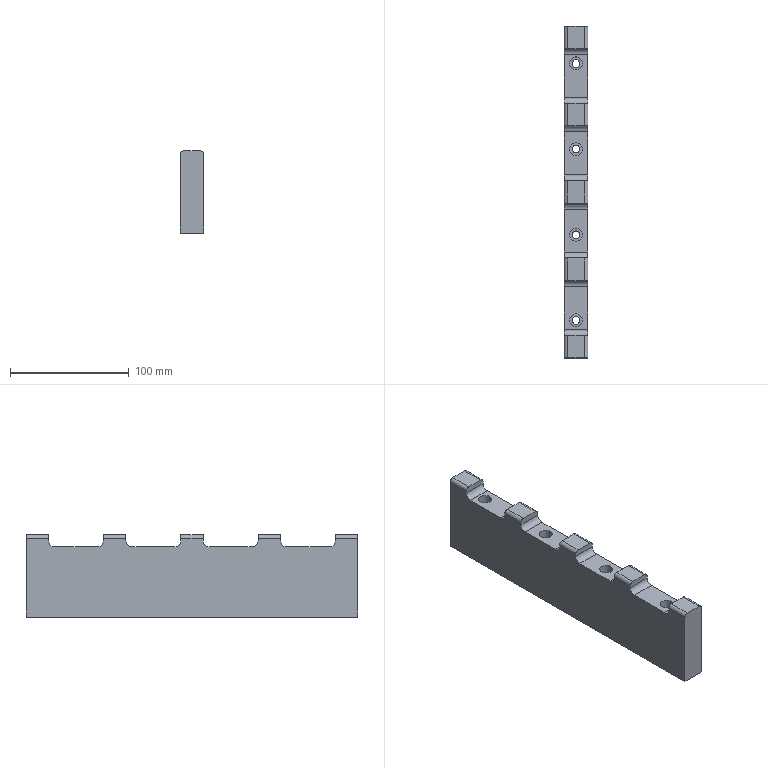CAM job | NX | 3+2 milling | part box 20 x 279 x 69 mm | stock box 25 x 284 x 70 mm
Tools:
number,name,description,diameter,corner_radius,flute_length,length,flutes
9,D10,平底铣刀-粗,10.0,0.0,35.0,75.0,2
10,D10-J,平底铣刀-精,10.0,0.0,35.0,75.0,2
17,D6R0.5,圆鼻刀-粗,6.0,0.5,50.0,75.0,2
1,D80R0.8飞刀,圆鼻刀-粗,80.0,0.8,50.0,75.0,2
1,D80R0.8飞刀-J,圆鼻刀-精,80.0,0.8,50.0,75.0,2
2,D6倒角刀,倒角刀,6.0,0.0,3.0,25.0,2
Operations:
program,operation,operation_type,tool,method,geometry_group,spindle_rpm,surface_speed,feed_per_tooth,feed_cut,feed_plunge,cut_length_mm,path_length_mm,cut_time_min,machine_time_min
B,底壁铣飞面一刀开粗_COPY,VolumeBased25DMillingOperation,D80R0.8飞刀,分层开粗-切深K-步距G,W-B,5000.0,1256.637,0.3,3000.0,100.0,3484.746,7108.966,1.162,1.524
B,底壁铣飞面一刀精光_COPY,VolumeBased25DMillingOperation,D80R0.8飞刀-J,侧刃精光-切深K-步距G,W-B,5000.0,1256.637,0.1,1000.0,100.0,386.998,482.998,0.387,0.3966
B,平面去毛刺6X45L_COPY,SurfaceContour,D6倒角刀,爬面_倒角-切深0-步距G,W-B,6500.0,122.519,0.1154,1500.0,100.0,647.511,1363.137,0.4317,0.5032
B,等高精光往复爬面_COPY_COPY,ZLevelMilling,D6R0.5,等高爬面-切深K-步距G,W-B,7000.0,131.947,0.3214,4500.0,100.0,6205.288,6609.64,1.379,1.419
A,顶面,FaceMilling,D80R0.8飞刀,侧刃精光-切深K-步距G,W-A,5000.0,1256.637,0.1,1000.0,100.0,373.0,409.0,0.373,0.3766
A,型腔铣开粗-中_COPY,CavityMilling,D10,分层开粗-切深K-步距G,W-A,8000.0,251.32,0.25,4000.0,100.0,41614.969,57039.534,10.404,12.926
A,等高精光往复爬面_COPY,ZLevelMilling,D6R0.5,等高爬面-切深K-步距G,W-A,7000.0,131.947,0.3214,4500.0,100.0,6204.525,6601.145,1.379,1.418
A,仅选体,SurfaceContour,D6倒角刀,METHOD,W-A,8000.0,150.796,0.1875,3000.0,100.0,669.422,1385.818,0.2231,0.2948
A,外形半精_2,VolumeBased25DMillingOperation,D10-J,METHOD,W-A,8000.0,251.327,0.0625,1000.0,100.0,1590.412,1732.427,1.59,1.605